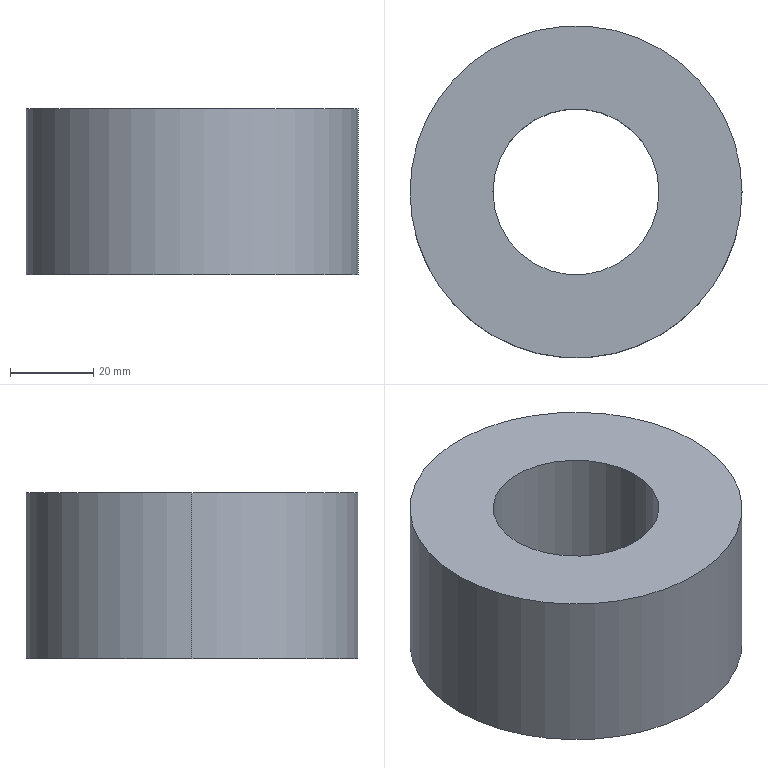Part | SolidWorks | features Extrusion 1 | 1 solid | 6 faces | box 80 x 80 x 40 mm | volume 150796 mm3 | cylinder 4 | plane 2 | commonest cylinder face diameters 40 x2 80 x2
STEP:
#1=CARTESIAN_POINT('',(-20.,0.,20.));
#2=VERTEX_POINT('',#1);
#3=CARTESIAN_POINT('',(20.,0.,20.));
#4=VERTEX_POINT('',#3);
#5=CARTESIAN_POINT('',(0.,0.,20.));
#6=DIRECTION('',(0.,0.,1.));
#7=DIRECTION('',(1.,0.,0.));
#8=AXIS2_PLACEMENT_3D('',#5,#6,#7);
#9=CIRCLE('',#8,20.);
#10=EDGE_CURVE('',#2,#4,#9,.T.);
#11=ORIENTED_EDGE('',*,*,#10,.T.);
#12=CARTESIAN_POINT('',(20.,0.,-20.));
#13=VERTEX_POINT('',#12);
#14=CARTESIAN_POINT('',(20.,0.,20.));
#15=DIRECTION('',(0.,0.,-1.));
#16=VECTOR('',#15,1000.);
#17=LINE('',#14,#16);
#18=EDGE_CURVE('',#4,#13,#17,.T.);
#19=ORIENTED_EDGE('',*,*,#18,.T.);
#20=CARTESIAN_POINT('',(-20.,0.,-20.));
#21=VERTEX_POINT('',#20);
#22=CARTESIAN_POINT('',(0.,0.,-20.));
#23=DIRECTION('',(0.,0.,1.));
#24=DIRECTION('',(1.,0.,0.));
#25=AXIS2_PLACEMENT_3D('',#22,#23,#24);
#26=CIRCLE('',#25,20.);
#27=EDGE_CURVE('',#21,#13,#26,.T.);
#28=ORIENTED_EDGE('',*,*,#27,.F.);
#29=CARTESIAN_POINT('',(-20.,0.,20.));
#30=DIRECTION('',(0.,0.,-1.));
#31=VECTOR('',#30,1000.);
#32=LINE('',#29,#31);
#33=EDGE_CURVE('',#2,#21,#32,.T.);
#34=ORIENTED_EDGE('',*,*,#33,.F.);
#35=EDGE_LOOP('',(#11,#19,#28,#34));
#36=FACE_OUTER_BOUND('',#35,.T.);
#37=CARTESIAN_POINT('',(0.,0.,20.));
#38=DIRECTION('',(0.,0.,-1.));
#39=DIRECTION('',(-1.,0.,0.));
#40=AXIS2_PLACEMENT_3D('',#37,#38,#39);
#41=CYLINDRICAL_SURFACE('',#40,20.);
#42=ADVANCED_FACE('',(#36),#41,.F.);
#43=CARTESIAN_POINT('',(40.,0.,20.));
#44=VERTEX_POINT('',#43);
#45=CARTESIAN_POINT('',(-40.,0.,20.));
#46=VERTEX_POINT('',#45);
#47=CARTESIAN_POINT('',(0.,0.,20.));
#48=DIRECTION('',(0.,0.,1.));
#49=DIRECTION('',(1.,0.,0.));
#50=AXIS2_PLACEMENT_3D('',#47,#48,#49);
#51=CIRCLE('',#50,40.);
#52=EDGE_CURVE('',#44,#46,#51,.T.);
#53=ORIENTED_EDGE('',*,*,#52,.F.);
#54=CARTESIAN_POINT('',(40.,0.,-20.));
#55=VERTEX_POINT('',#54);
#56=CARTESIAN_POINT('',(40.,0.,20.));
#57=DIRECTION('',(0.,0.,-1.));
#58=VECTOR('',#57,1000.);
#59=LINE('',#56,#58);
#60=EDGE_CURVE('',#44,#55,#59,.T.);
#61=ORIENTED_EDGE('',*,*,#60,.T.);
#62=CARTESIAN_POINT('',(-40.,0.,-20.));
#63=VERTEX_POINT('',#62);
#64=CARTESIAN_POINT('',(0.,0.,-20.));
#65=DIRECTION('',(0.,0.,1.));
#66=DIRECTION('',(1.,0.,0.));
#67=AXIS2_PLACEMENT_3D('',#64,#65,#66);
#68=CIRCLE('',#67,40.);
#69=EDGE_CURVE('',#55,#63,#68,.T.);
#70=ORIENTED_EDGE('',*,*,#69,.T.);
#71=CARTESIAN_POINT('',(-40.,0.,20.));
#72=DIRECTION('',(0.,0.,-1.));
#73=VECTOR('',#72,1000.);
#74=LINE('',#71,#73);
#75=EDGE_CURVE('',#46,#63,#74,.T.);
#76=ORIENTED_EDGE('',*,*,#75,.F.);
#77=EDGE_LOOP('',(#53,#61,#70,#76));
#78=FACE_OUTER_BOUND('',#77,.T.);
#79=CARTESIAN_POINT('',(0.,0.,20.));
#80=DIRECTION('',(0.,0.,-1.));
#81=DIRECTION('',(-1.,0.,0.));
#82=AXIS2_PLACEMENT_3D('',#79,#80,#81);
#83=CYLINDRICAL_SURFACE('',#82,40.);
#84=ADVANCED_FACE('',(#78),#83,.T.);
#85=CARTESIAN_POINT('',(0.,0.,20.));
#86=DIRECTION('',(0.,0.,1.));
#87=DIRECTION('',(1.,0.,0.));
#88=AXIS2_PLACEMENT_3D('',#85,#86,#87);
#89=CIRCLE('',#88,40.);
#90=EDGE_CURVE('',#46,#44,#89,.T.);
#91=ORIENTED_EDGE('',*,*,#90,.T.);
#92=ORIENTED_EDGE('',*,*,#52,.T.);
#93=EDGE_LOOP('',(#91,#92));
#94=FACE_OUTER_BOUND('',#93,.T.);
#95=ORIENTED_EDGE('',*,*,#10,.F.);
#96=CARTESIAN_POINT('',(0.,0.,20.));
#97=DIRECTION('',(0.,0.,1.));
#98=DIRECTION('',(1.,0.,0.));
#99=AXIS2_PLACEMENT_3D('',#96,#97,#98);
#100=CIRCLE('',#99,20.);
#101=EDGE_CURVE('',#4,#2,#100,.T.);
#102=ORIENTED_EDGE('',*,*,#101,.F.);
#103=EDGE_LOOP('',(#95,#102));
#104=FACE_BOUND('',#103,.T.);
#105=CARTESIAN_POINT('',(0.,0.,20.));
#106=DIRECTION('',(0.,0.,1.));
#107=DIRECTION('',(1.,0.,0.));
#108=AXIS2_PLACEMENT_3D('',#105,#106,#107);
#109=PLANE('',#108);
#110=ADVANCED_FACE('',(#94,#104),#109,.T.);
#111=CARTESIAN_POINT('',(0.,0.,-20.));
#112=DIRECTION('',(0.,0.,1.));
#113=DIRECTION('',(1.,0.,0.));
#114=AXIS2_PLACEMENT_3D('',#111,#112,#113);
#115=CIRCLE('',#114,40.);
#116=EDGE_CURVE('',#63,#55,#115,.T.);
#117=ORIENTED_EDGE('',*,*,#116,.F.);
#118=ORIENTED_EDGE('',*,*,#69,.F.);
#119=EDGE_LOOP('',(#117,#118));
#120=FACE_OUTER_BOUND('',#119,.T.);
#121=ORIENTED_EDGE('',*,*,#27,.T.);
#122=CARTESIAN_POINT('',(0.,0.,-20.));
#123=DIRECTION('',(0.,0.,1.));
#124=DIRECTION('',(1.,0.,0.));
#125=AXIS2_PLACEMENT_3D('',#122,#123,#124);
#126=CIRCLE('',#125,20.);
#127=EDGE_CURVE('',#13,#21,#126,.T.);
#128=ORIENTED_EDGE('',*,*,#127,.T.);
#129=EDGE_LOOP('',(#121,#128));
#130=FACE_BOUND('',#129,.T.);
#131=CARTESIAN_POINT('',(0.,0.,-20.));
#132=DIRECTION('',(0.,0.,1.));
#133=DIRECTION('',(1.,0.,0.));
#134=AXIS2_PLACEMENT_3D('',#131,#132,#133);
#135=PLANE('',#134);
#136=ADVANCED_FACE('',(#120,#130),#135,.F.);
#137=ORIENTED_EDGE('',*,*,#60,.F.);
#138=ORIENTED_EDGE('',*,*,#90,.F.);
#139=ORIENTED_EDGE('',*,*,#75,.T.);
#140=ORIENTED_EDGE('',*,*,#116,.T.);
#141=EDGE_LOOP('',(#137,#138,#139,#140));
#142=FACE_OUTER_BOUND('',#141,.T.);
#143=CARTESIAN_POINT('',(0.,0.,20.));
#144=DIRECTION('',(0.,0.,-1.));
#145=DIRECTION('',(-1.,0.,0.));
#146=AXIS2_PLACEMENT_3D('',#143,#144,#145);
#147=CYLINDRICAL_SURFACE('',#146,40.);
#148=ADVANCED_FACE('',(#142),#147,.T.);
#149=ORIENTED_EDGE('',*,*,#18,.F.);
#150=ORIENTED_EDGE('',*,*,#101,.T.);
#151=ORIENTED_EDGE('',*,*,#33,.T.);
#152=ORIENTED_EDGE('',*,*,#127,.F.);
#153=EDGE_LOOP('',(#149,#150,#151,#152));
#154=FACE_OUTER_BOUND('',#153,.T.);
#155=CARTESIAN_POINT('',(0.,0.,20.));
#156=DIRECTION('',(0.,0.,-1.));
#157=DIRECTION('',(-1.,0.,0.));
#158=AXIS2_PLACEMENT_3D('',#155,#156,#157);
#159=CYLINDRICAL_SURFACE('',#158,20.);
#160=ADVANCED_FACE('',(#154),#159,.F.);
#161=CLOSED_SHELL('',(#42,#84,#110,#136,#148,#160));
#162=MANIFOLD_SOLID_BREP('',#161);
#163=CARTESIAN_POINT('',(0.,0.,0.));
#164=DIRECTION('',(0.,0.,1.));
#165=DIRECTION('',(1.,0.,0.));
#166=AXIS2_PLACEMENT_3D('',#163,#164,#165);
#167=(LENGTH_UNIT()NAMED_UNIT(*)SI_UNIT(.MILLI.,.METRE.));
#168=UNCERTAINTY_MEASURE_WITH_UNIT(LENGTH_MEASURE(0.00001),#167,'','');
#169=(NAMED_UNIT(*)PLANE_ANGLE_UNIT()SI_UNIT($,.RADIAN.));
#170=(NAMED_UNIT(*)SI_UNIT($,.STERADIAN.)SOLID_ANGLE_UNIT());
#171=(GEOMETRIC_REPRESENTATION_CONTEXT(3)GLOBAL_UNCERTAINTY_ASSIGNED_CONTEXT((#168))GLOBAL_UNIT_ASSIGNED_CONTEXT((#167,#169,#170))REPRESENTATION_CONTEXT('',''));
#172=ADVANCED_BREP_SHAPE_REPRESENTATION('',(#162,#166),#171);